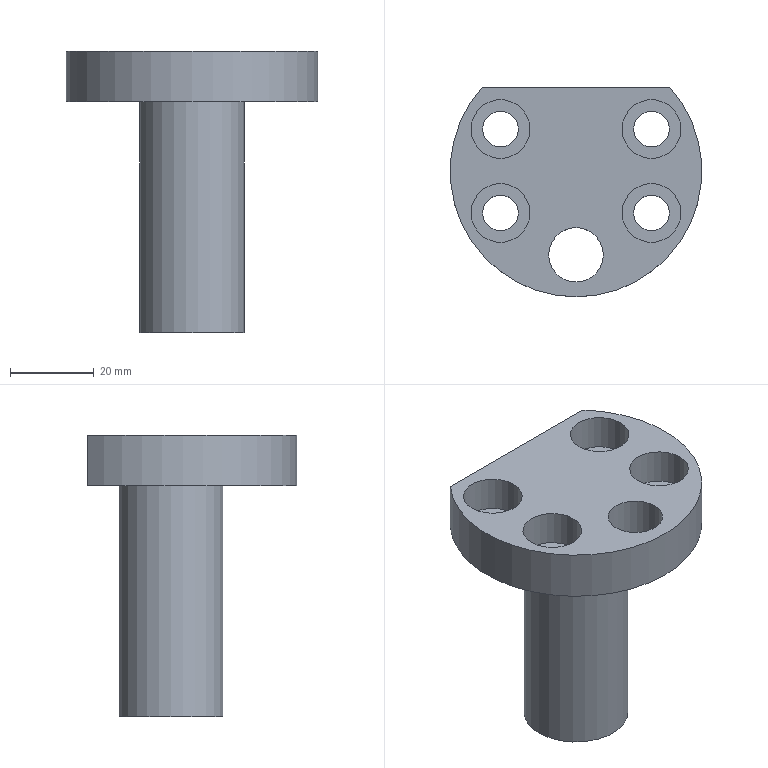CAM job | NX | 3-axis milling, drilling | part box 60 x 50 x 67 mm | stock box 60 x 60 x 67 mm
Tools:
number,name,description,diameter,corner_radius,flute_length,length,flutes
1,ZXZ,Milling Tool-5 Parameters,6.0,0.0,50.0,75.0,2
7,D6A45,Milling Tool-5 Parameters,6.0,0.0,3.0,3.0,2
2,8.5ZT,Drilling Tool,8.5,0.0,35.0,50.0,2
3,13.0ZT,Drilling Tool,13.0,0.0,35.0,50.0,2
10,D10,Milling Tool-5 Parameters,10.0,0.0,50.0,75.0,2
Operations:
program,operation,operation_type,tool,method,geometry_group,spindle_rpm,surface_speed,feed_per_tooth,feed_cut,feed_plunge,cut_length_mm,path_length_mm,cut_time_min,machine_time_min
1,DRILLING,Operation,ZXZ,METHOD,A,3000.0,56.0,0.0333,200.0,0.0,20.0,194.065,0.1,0.1174
1,DRILLING_COPY,Operation,8.5ZT,METHOD,A,1200.0,32.0,0.05,120.0,0.0,76.215,313.903,0.6351,0.6589
1,DRILLING_COPY_COPY,Operation,13.0ZT,METHOD,A,600.0,24.0,0.1,120.0,0.0,20.406,100.811,0.17,0.1781
1,HOLE_MILLING,CylinderMilling,D10,METHOD,A,3000.0,94.0,0.3333,2000.0,100.0,2132.028,2480.028,1.066,1.101
1,ZLEVEL_PROFILE_1_COPY_1,ZLevelMilling,D6A45,METHOD,A,7500.0,141.0,0.0667,1000.0,100.0,217.445,690.505,0.2174,0.2648